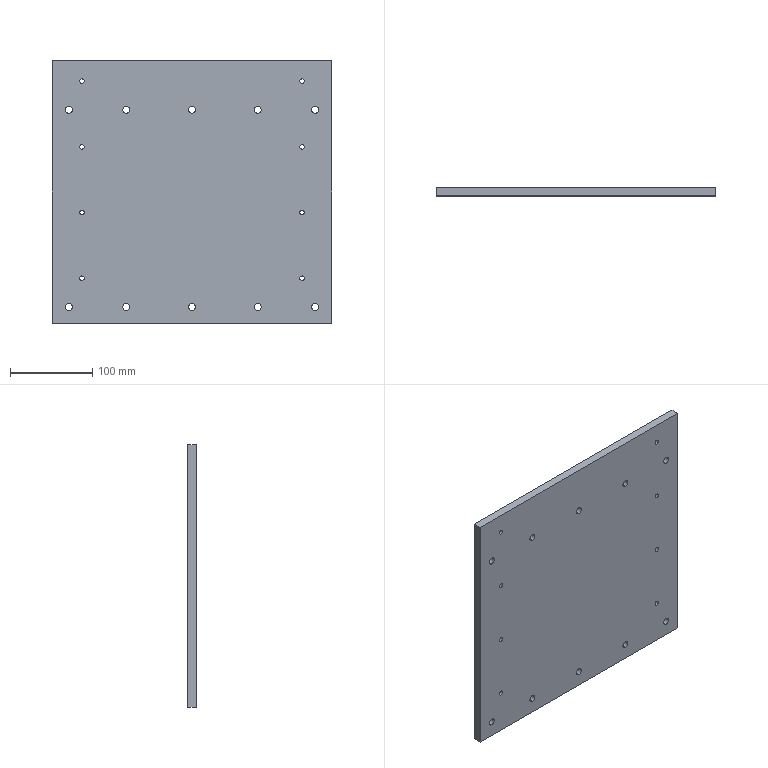Part | STEP file | PN_0001 (support block) | 1 solid | 66 faces | box 340 x 10 x 320 mm | volume 1077927 mm3 | cylinder 52 | plane 14 | commonest cylinder face diameters 8.5 x20 5.5 x16 10 x16